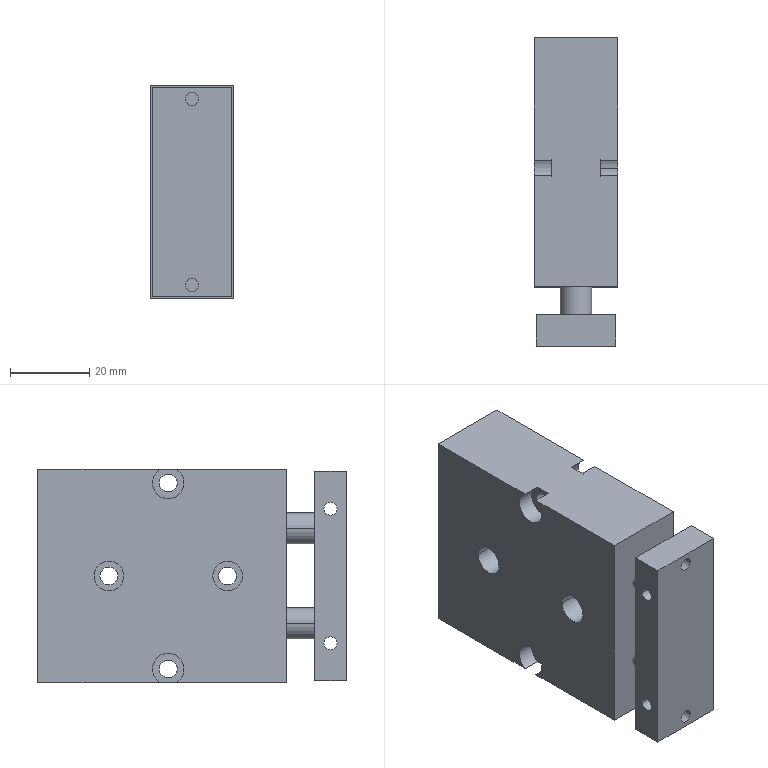Part | STEP file | Cylinder TN-16-10-S Retract | 2 solids | 56 faces | box 21 x 78 x 54 mm | volume 81436 mm3 | cylinder 34 | plane 22 | commonest cylinder face diameters 8 x10 3.3 x8 4.5 x8 7.5 x8